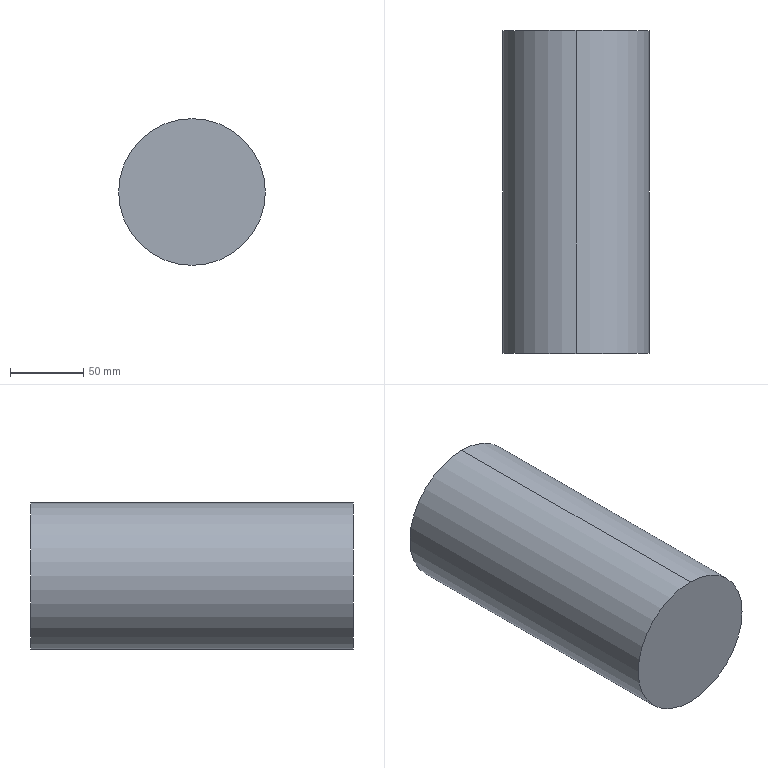Part | SolidWorks | features BaseBody 1 | 1 solid | 4 faces | box 100 x 220 x 100 mm | volume 1727876 mm3 | cylinder 2 | plane 2 | commonest cylinder face diameters 100 x2
STEP:
#1=CARTESIAN_POINT('',(0.,220.,-46.195));
#2=VERTEX_POINT('',#1);
#3=CARTESIAN_POINT('',(0.,220.,53.805));
#4=VERTEX_POINT('',#3);
#5=CARTESIAN_POINT('',(0.,220.,3.805));
#6=DIRECTION('',(0.,-1.,0.));
#7=DIRECTION('',(0.,0.,-1.));
#8=AXIS2_PLACEMENT_3D('',#5,#6,#7);
#9=CIRCLE('',#8,50.);
#10=EDGE_CURVE('',#2,#4,#9,.T.);
#11=ORIENTED_EDGE('',*,*,#10,.T.);
#12=CARTESIAN_POINT('',(0.,0.,53.805));
#13=VERTEX_POINT('',#12);
#14=CARTESIAN_POINT('',(0.,220.,53.805));
#15=DIRECTION('',(0.,-1.,0.));
#16=VECTOR('',#15,1000.);
#17=LINE('',#14,#16);
#18=EDGE_CURVE('',#4,#13,#17,.T.);
#19=ORIENTED_EDGE('',*,*,#18,.T.);
#20=CARTESIAN_POINT('',(0.,0.,-46.195));
#21=VERTEX_POINT('',#20);
#22=CARTESIAN_POINT('',(0.,0.,3.805));
#23=DIRECTION('',(0.,1.,0.));
#24=DIRECTION('',(0.,0.,-1.));
#25=AXIS2_PLACEMENT_3D('',#22,#23,#24);
#26=CIRCLE('',#25,50.);
#27=EDGE_CURVE('',#13,#21,#26,.T.);
#28=ORIENTED_EDGE('',*,*,#27,.T.);
#29=CARTESIAN_POINT('',(0.,220.,-46.195));
#30=DIRECTION('',(0.,-1.,0.));
#31=VECTOR('',#30,1000.);
#32=LINE('',#29,#31);
#33=EDGE_CURVE('',#2,#21,#32,.T.);
#34=ORIENTED_EDGE('',*,*,#33,.F.);
#35=EDGE_LOOP('',(#11,#19,#28,#34));
#36=FACE_OUTER_BOUND('',#35,.T.);
#37=CARTESIAN_POINT('',(0.,220.,3.805));
#38=DIRECTION('',(0.,-1.,0.));
#39=DIRECTION('',(0.,0.,-1.));
#40=AXIS2_PLACEMENT_3D('',#37,#38,#39);
#41=CYLINDRICAL_SURFACE('',#40,50.);
#42=ADVANCED_FACE('',(#36),#41,.T.);
#43=ORIENTED_EDGE('',*,*,#18,.F.);
#44=CARTESIAN_POINT('',(0.,220.,3.805));
#45=DIRECTION('',(0.,-1.,0.));
#46=DIRECTION('',(0.,0.,-1.));
#47=AXIS2_PLACEMENT_3D('',#44,#45,#46);
#48=CIRCLE('',#47,50.);
#49=EDGE_CURVE('',#4,#2,#48,.T.);
#50=ORIENTED_EDGE('',*,*,#49,.T.);
#51=ORIENTED_EDGE('',*,*,#33,.T.);
#52=CARTESIAN_POINT('',(0.,0.,3.805));
#53=DIRECTION('',(0.,1.,0.));
#54=DIRECTION('',(0.,0.,-1.));
#55=AXIS2_PLACEMENT_3D('',#52,#53,#54);
#56=CIRCLE('',#55,50.);
#57=EDGE_CURVE('',#21,#13,#56,.T.);
#58=ORIENTED_EDGE('',*,*,#57,.T.);
#59=EDGE_LOOP('',(#43,#50,#51,#58));
#60=FACE_OUTER_BOUND('',#59,.T.);
#61=CARTESIAN_POINT('',(0.,220.,3.805));
#62=DIRECTION('',(0.,-1.,0.));
#63=DIRECTION('',(0.,0.,-1.));
#64=AXIS2_PLACEMENT_3D('',#61,#62,#63);
#65=CYLINDRICAL_SURFACE('',#64,50.);
#66=ADVANCED_FACE('',(#60),#65,.T.);
#67=ORIENTED_EDGE('',*,*,#57,.F.);
#68=ORIENTED_EDGE('',*,*,#27,.F.);
#69=EDGE_LOOP('',(#67,#68));
#70=FACE_OUTER_BOUND('',#69,.T.);
#71=CARTESIAN_POINT('',(0.,0.,3.805));
#72=DIRECTION('',(0.,1.,0.));
#73=DIRECTION('',(0.,0.,1.));
#74=AXIS2_PLACEMENT_3D('',#71,#72,#73);
#75=PLANE('',#74);
#76=ADVANCED_FACE('',(#70),#75,.F.);
#77=ORIENTED_EDGE('',*,*,#10,.F.);
#78=ORIENTED_EDGE('',*,*,#49,.F.);
#79=EDGE_LOOP('',(#77,#78));
#80=FACE_OUTER_BOUND('',#79,.T.);
#81=CARTESIAN_POINT('',(0.,220.,3.805));
#82=DIRECTION('',(0.,1.,0.));
#83=DIRECTION('',(0.,0.,1.));
#84=AXIS2_PLACEMENT_3D('',#81,#82,#83);
#85=PLANE('',#84);
#86=ADVANCED_FACE('',(#80),#85,.T.);
#87=CLOSED_SHELL('',(#42,#66,#76,#86));
#88=MANIFOLD_SOLID_BREP('',#87);
#89=CARTESIAN_POINT('',(0.,0.,0.));
#90=DIRECTION('',(0.,0.,1.));
#91=DIRECTION('',(1.,0.,0.));
#92=AXIS2_PLACEMENT_3D('',#89,#90,#91);
#93=(LENGTH_UNIT()NAMED_UNIT(*)SI_UNIT(.MILLI.,.METRE.));
#94=UNCERTAINTY_MEASURE_WITH_UNIT(LENGTH_MEASURE(0.00001),#93,'','');
#95=(NAMED_UNIT(*)PLANE_ANGLE_UNIT()SI_UNIT($,.RADIAN.));
#96=(NAMED_UNIT(*)SI_UNIT($,.STERADIAN.)SOLID_ANGLE_UNIT());
#97=(GEOMETRIC_REPRESENTATION_CONTEXT(3)GLOBAL_UNCERTAINTY_ASSIGNED_CONTEXT((#94))GLOBAL_UNIT_ASSIGNED_CONTEXT((#93,#95,#96))REPRESENTATION_CONTEXT('',''));
#98=ADVANCED_BREP_SHAPE_REPRESENTATION('',(#88,#92),#97);